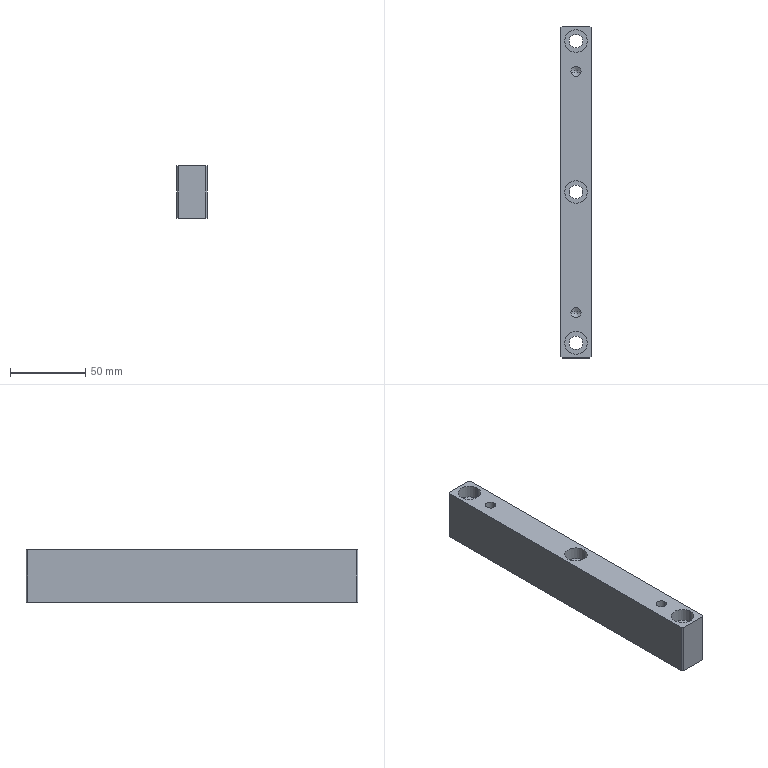Part | SolidWorks | features HoleWzd 2, Chamfer 1, Extrusion 1 | 1 solid | 33 faces | box 20 x 220 x 35 mm | volume 142848 mm3 | cylinder 16 | plane 13 | cone 4 | commonest cylinder face diameters 9 x6 15 x6 6.8 x4
STEP:
#1=CARTESIAN_POINT('',(-3.4,80.,-2.25));
#2=VERTEX_POINT('',#1);
#3=CARTESIAN_POINT('',(3.4,80.,-2.25));
#4=VERTEX_POINT('',#3);
#5=CARTESIAN_POINT('',(0.,80.,-2.25));
#6=DIRECTION('',(0.,0.,1.));
#7=DIRECTION('',(1.,0.,0.));
#8=AXIS2_PLACEMENT_3D('',#5,#6,#7);
#9=CIRCLE('',#8,3.4);
#10=EDGE_CURVE('',#2,#4,#9,.T.);
#11=ORIENTED_EDGE('',*,*,#10,.F.);
#12=CARTESIAN_POINT('',(-3.4,80.,17.5));
#13=VERTEX_POINT('',#12);
#14=CARTESIAN_POINT('',(-3.4,80.,17.5));
#15=DIRECTION('',(0.,0.,1.));
#16=VECTOR('',#15,1000.);
#17=LINE('',#14,#16);
#18=EDGE_CURVE('',#2,#13,#17,.T.);
#19=ORIENTED_EDGE('',*,*,#18,.T.);
#20=CARTESIAN_POINT('',(3.4,80.,17.5));
#21=VERTEX_POINT('',#20);
#22=CARTESIAN_POINT('',(0.,80.,17.5));
#23=DIRECTION('',(0.,0.,1.));
#24=DIRECTION('',(1.,0.,0.));
#25=AXIS2_PLACEMENT_3D('',#22,#23,#24);
#26=CIRCLE('',#25,3.4);
#27=EDGE_CURVE('',#13,#21,#26,.T.);
#28=ORIENTED_EDGE('',*,*,#27,.T.);
#29=CARTESIAN_POINT('',(3.4,80.,17.5));
#30=DIRECTION('',(0.,0.,1.));
#31=VECTOR('',#30,1000.);
#32=LINE('',#29,#31);
#33=EDGE_CURVE('',#4,#21,#32,.T.);
#34=ORIENTED_EDGE('',*,*,#33,.F.);
#35=EDGE_LOOP('',(#11,#19,#28,#34));
#36=FACE_OUTER_BOUND('',#35,.T.);
#37=CARTESIAN_POINT('',(0.,80.,17.5));
#38=DIRECTION('',(0.,0.,1.));
#39=DIRECTION('',(1.,0.,0.));
#40=AXIS2_PLACEMENT_3D('',#37,#38,#39);
#41=CYLINDRICAL_SURFACE('',#40,3.4);
#42=ADVANCED_FACE('',(#36),#41,.F.);
#43=CARTESIAN_POINT('',(0.,80.,-4.293));
#44=VERTEX_POINT('',#43);
#45=CARTESIAN_POINT('',(3.4,80.,-2.25));
#46=DIRECTION('',(0.8572,0.,0.515));
#47=VECTOR('',#46,1000.);
#48=LINE('',#45,#47);
#49=EDGE_CURVE('',#44,#4,#48,.T.);
#50=ORIENTED_EDGE('',*,*,#49,.F.);
#51=CARTESIAN_POINT('',(-3.4,80.,-2.25));
#52=DIRECTION('',(-0.8572,0.,0.515));
#53=VECTOR('',#52,1000.);
#54=LINE('',#51,#53);
#55=EDGE_CURVE('',#44,#2,#54,.T.);
#56=ORIENTED_EDGE('',*,*,#55,.T.);
#57=ORIENTED_EDGE('',*,*,#10,.T.);
#58=EDGE_LOOP('',(#50,#56,#57));
#59=FACE_OUTER_BOUND('',#58,.T.);
#60=CARTESIAN_POINT('',(0.,80.,-2.25));
#61=DIRECTION('',(0.,0.,1.));
#62=DIRECTION('',(1.,0.,0.));
#63=AXIS2_PLACEMENT_3D('',#60,#61,#62);
#64=CONICAL_SURFACE('',#63,3.4,1.03);
#65=ADVANCED_FACE('',(#59),#64,.F.);
#66=CARTESIAN_POINT('',(-3.4,-80.,-2.25));
#67=VERTEX_POINT('',#66);
#68=CARTESIAN_POINT('',(3.4,-80.,-2.25));
#69=VERTEX_POINT('',#68);
#70=CARTESIAN_POINT('',(0.,-80.,-2.25));
#71=DIRECTION('',(0.,0.,1.));
#72=DIRECTION('',(1.,0.,0.));
#73=AXIS2_PLACEMENT_3D('',#70,#71,#72);
#74=CIRCLE('',#73,3.4);
#75=EDGE_CURVE('',#67,#69,#74,.T.);
#76=ORIENTED_EDGE('',*,*,#75,.F.);
#77=CARTESIAN_POINT('',(-3.4,-80.,17.5));
#78=VERTEX_POINT('',#77);
#79=CARTESIAN_POINT('',(-3.4,-80.,17.5));
#80=DIRECTION('',(0.,0.,1.));
#81=VECTOR('',#80,1000.);
#82=LINE('',#79,#81);
#83=EDGE_CURVE('',#67,#78,#82,.T.);
#84=ORIENTED_EDGE('',*,*,#83,.T.);
#85=CARTESIAN_POINT('',(3.4,-80.,17.5));
#86=VERTEX_POINT('',#85);
#87=CARTESIAN_POINT('',(0.,-80.,17.5));
#88=DIRECTION('',(0.,0.,1.));
#89=DIRECTION('',(1.,0.,0.));
#90=AXIS2_PLACEMENT_3D('',#87,#88,#89);
#91=CIRCLE('',#90,3.4);
#92=EDGE_CURVE('',#78,#86,#91,.T.);
#93=ORIENTED_EDGE('',*,*,#92,.T.);
#94=CARTESIAN_POINT('',(3.4,-80.,17.5));
#95=DIRECTION('',(0.,0.,1.));
#96=VECTOR('',#95,1000.);
#97=LINE('',#94,#96);
#98=EDGE_CURVE('',#69,#86,#97,.T.);
#99=ORIENTED_EDGE('',*,*,#98,.F.);
#100=EDGE_LOOP('',(#76,#84,#93,#99));
#101=FACE_OUTER_BOUND('',#100,.T.);
#102=CARTESIAN_POINT('',(0.,-80.,17.5));
#103=DIRECTION('',(0.,0.,1.));
#104=DIRECTION('',(1.,0.,0.));
#105=AXIS2_PLACEMENT_3D('',#102,#103,#104);
#106=CYLINDRICAL_SURFACE('',#105,3.4);
#107=ADVANCED_FACE('',(#101),#106,.F.);
#108=CARTESIAN_POINT('',(0.,-80.,-4.293));
#109=VERTEX_POINT('',#108);
#110=CARTESIAN_POINT('',(3.4,-80.,-2.25));
#111=DIRECTION('',(0.8572,0.,0.515));
#112=VECTOR('',#111,1000.);
#113=LINE('',#110,#112);
#114=EDGE_CURVE('',#109,#69,#113,.T.);
#115=ORIENTED_EDGE('',*,*,#114,.F.);
#116=CARTESIAN_POINT('',(-3.4,-80.,-2.25));
#117=DIRECTION('',(-0.8572,0.,0.515));
#118=VECTOR('',#117,1000.);
#119=LINE('',#116,#118);
#120=EDGE_CURVE('',#109,#67,#119,.T.);
#121=ORIENTED_EDGE('',*,*,#120,.T.);
#122=ORIENTED_EDGE('',*,*,#75,.T.);
#123=EDGE_LOOP('',(#115,#121,#122));
#124=FACE_OUTER_BOUND('',#123,.T.);
#125=CARTESIAN_POINT('',(0.,-80.,-2.25));
#126=DIRECTION('',(0.,0.,1.));
#127=DIRECTION('',(1.,0.,0.));
#128=AXIS2_PLACEMENT_3D('',#125,#126,#127);
#129=CONICAL_SURFACE('',#128,3.4,1.03);
#130=ADVANCED_FACE('',(#124),#129,.F.);
#131=CARTESIAN_POINT('',(-7.5,100.,8.9));
#132=VERTEX_POINT('',#131);
#133=CARTESIAN_POINT('',(7.5,100.,8.9));
#134=VERTEX_POINT('',#133);
#135=CARTESIAN_POINT('',(0.,100.,8.9));
#136=DIRECTION('',(0.,0.,1.));
#137=DIRECTION('',(1.,0.,0.));
#138=AXIS2_PLACEMENT_3D('',#135,#136,#137);
#139=CIRCLE('',#138,7.5);
#140=EDGE_CURVE('',#132,#134,#139,.T.);
#141=ORIENTED_EDGE('',*,*,#140,.F.);
#142=CARTESIAN_POINT('',(-7.5,100.,17.5));
#143=VERTEX_POINT('',#142);
#144=CARTESIAN_POINT('',(-7.5,100.,17.5));
#145=DIRECTION('',(0.,0.,1.));
#146=VECTOR('',#145,1000.);
#147=LINE('',#144,#146);
#148=EDGE_CURVE('',#132,#143,#147,.T.);
#149=ORIENTED_EDGE('',*,*,#148,.T.);
#150=CARTESIAN_POINT('',(7.5,100.,17.5));
#151=VERTEX_POINT('',#150);
#152=CARTESIAN_POINT('',(0.,100.,17.5));
#153=DIRECTION('',(0.,0.,1.));
#154=DIRECTION('',(1.,0.,0.));
#155=AXIS2_PLACEMENT_3D('',#152,#153,#154);
#156=CIRCLE('',#155,7.5);
#157=EDGE_CURVE('',#143,#151,#156,.T.);
#158=ORIENTED_EDGE('',*,*,#157,.T.);
#159=CARTESIAN_POINT('',(7.5,100.,17.5));
#160=DIRECTION('',(0.,0.,1.));
#161=VECTOR('',#160,1000.);
#162=LINE('',#159,#161);
#163=EDGE_CURVE('',#134,#151,#162,.T.);
#164=ORIENTED_EDGE('',*,*,#163,.F.);
#165=EDGE_LOOP('',(#141,#149,#158,#164));
#166=FACE_OUTER_BOUND('',#165,.T.);
#167=CARTESIAN_POINT('',(0.,100.,17.5));
#168=DIRECTION('',(0.,0.,1.));
#169=DIRECTION('',(1.,0.,0.));
#170=AXIS2_PLACEMENT_3D('',#167,#168,#169);
#171=CYLINDRICAL_SURFACE('',#170,7.5);
#172=ADVANCED_FACE('',(#166),#171,.F.);
#173=CARTESIAN_POINT('',(-4.5,100.,-17.5));
#174=VERTEX_POINT('',#173);
#175=CARTESIAN_POINT('',(4.5,100.,-17.5));
#176=VERTEX_POINT('',#175);
#177=CARTESIAN_POINT('',(0.,100.,-17.5));
#178=DIRECTION('',(0.,0.,1.));
#179=DIRECTION('',(1.,0.,0.));
#180=AXIS2_PLACEMENT_3D('',#177,#178,#179);
#181=CIRCLE('',#180,4.5);
#182=EDGE_CURVE('',#174,#176,#181,.T.);
#183=ORIENTED_EDGE('',*,*,#182,.F.);
#184=CARTESIAN_POINT('',(-4.5,100.,8.9));
#185=VERTEX_POINT('',#184);
#186=CARTESIAN_POINT('',(-4.5,100.,17.5));
#187=DIRECTION('',(0.,0.,1.));
#188=VECTOR('',#187,1000.);
#189=LINE('',#186,#188);
#190=EDGE_CURVE('',#174,#185,#189,.T.);
#191=ORIENTED_EDGE('',*,*,#190,.T.);
#192=CARTESIAN_POINT('',(4.5,100.,8.9));
#193=VERTEX_POINT('',#192);
#194=CARTESIAN_POINT('',(0.,100.,8.9));
#195=DIRECTION('',(0.,0.,1.));
#196=DIRECTION('',(1.,0.,0.));
#197=AXIS2_PLACEMENT_3D('',#194,#195,#196);
#198=CIRCLE('',#197,4.5);
#199=EDGE_CURVE('',#185,#193,#198,.T.);
#200=ORIENTED_EDGE('',*,*,#199,.T.);
#201=CARTESIAN_POINT('',(4.5,100.,17.5));
#202=DIRECTION('',(0.,0.,1.));
#203=VECTOR('',#202,1000.);
#204=LINE('',#201,#203);
#205=EDGE_CURVE('',#176,#193,#204,.T.);
#206=ORIENTED_EDGE('',*,*,#205,.F.);
#207=EDGE_LOOP('',(#183,#191,#200,#206));
#208=FACE_OUTER_BOUND('',#207,.T.);
#209=CARTESIAN_POINT('',(0.,100.,17.5));
#210=DIRECTION('',(0.,0.,1.));
#211=DIRECTION('',(1.,0.,0.));
#212=AXIS2_PLACEMENT_3D('',#209,#210,#211);
#213=CYLINDRICAL_SURFACE('',#212,4.5);
#214=ADVANCED_FACE('',(#208),#213,.F.);
#215=CARTESIAN_POINT('',(-7.5,0.,8.9));
#216=VERTEX_POINT('',#215);
#217=CARTESIAN_POINT('',(7.5,0.,8.9));
#218=VERTEX_POINT('',#217);
#219=CARTESIAN_POINT('',(0.,0.,8.9));
#220=DIRECTION('',(0.,0.,1.));
#221=DIRECTION('',(1.,0.,0.));
#222=AXIS2_PLACEMENT_3D('',#219,#220,#221);
#223=CIRCLE('',#222,7.5);
#224=EDGE_CURVE('',#216,#218,#223,.T.);
#225=ORIENTED_EDGE('',*,*,#224,.F.);
#226=CARTESIAN_POINT('',(-7.5,0.,17.5));
#227=VERTEX_POINT('',#226);
#228=CARTESIAN_POINT('',(-7.5,0.,17.5));
#229=DIRECTION('',(0.,0.,1.));
#230=VECTOR('',#229,1000.);
#231=LINE('',#228,#230);
#232=EDGE_CURVE('',#216,#227,#231,.T.);
#233=ORIENTED_EDGE('',*,*,#232,.T.);
#234=CARTESIAN_POINT('',(7.5,0.,17.5));
#235=VERTEX_POINT('',#234);
#236=CARTESIAN_POINT('',(0.,0.,17.5));
#237=DIRECTION('',(0.,0.,1.));
#238=DIRECTION('',(1.,0.,0.));
#239=AXIS2_PLACEMENT_3D('',#236,#237,#238);
#240=CIRCLE('',#239,7.5);
#241=EDGE_CURVE('',#227,#235,#240,.T.);
#242=ORIENTED_EDGE('',*,*,#241,.T.);
#243=CARTESIAN_POINT('',(7.5,0.,17.5));
#244=DIRECTION('',(0.,0.,1.));
#245=VECTOR('',#244,1000.);
#246=LINE('',#243,#245);
#247=EDGE_CURVE('',#218,#235,#246,.T.);
#248=ORIENTED_EDGE('',*,*,#247,.F.);
#249=EDGE_LOOP('',(#225,#233,#242,#248));
#250=FACE_OUTER_BOUND('',#249,.T.);
#251=CARTESIAN_POINT('',(0.,0.,17.5));
#252=DIRECTION('',(0.,0.,1.));
#253=DIRECTION('',(1.,0.,0.));
#254=AXIS2_PLACEMENT_3D('',#251,#252,#253);
#255=CYLINDRICAL_SURFACE('',#254,7.5);
#256=ADVANCED_FACE('',(#250),#255,.F.);
#257=CARTESIAN_POINT('',(-4.5,0.,-17.5));
#258=VERTEX_POINT('',#257);
#259=CARTESIAN_POINT('',(4.5,0.,-17.5));
#260=VERTEX_POINT('',#259);
#261=CARTESIAN_POINT('',(0.,0.,-17.5));
#262=DIRECTION('',(0.,0.,1.));
#263=DIRECTION('',(1.,0.,0.));
#264=AXIS2_PLACEMENT_3D('',#261,#262,#263);
#265=CIRCLE('',#264,4.5);
#266=EDGE_CURVE('',#258,#260,#265,.T.);
#267=ORIENTED_EDGE('',*,*,#266,.F.);
#268=CARTESIAN_POINT('',(-4.5,0.,8.9));
#269=VERTEX_POINT('',#268);
#270=CARTESIAN_POINT('',(-4.5,0.,17.5));
#271=DIRECTION('',(0.,0.,1.));
#272=VECTOR('',#271,1000.);
#273=LINE('',#270,#272);
#274=EDGE_CURVE('',#258,#269,#273,.T.);
#275=ORIENTED_EDGE('',*,*,#274,.T.);
#276=CARTESIAN_POINT('',(4.5,0.,8.9));
#277=VERTEX_POINT('',#276);
#278=CARTESIAN_POINT('',(0.,0.,8.9));
#279=DIRECTION('',(0.,0.,1.));
#280=DIRECTION('',(1.,0.,0.));
#281=AXIS2_PLACEMENT_3D('',#278,#279,#280);
#282=CIRCLE('',#281,4.5);
#283=EDGE_CURVE('',#269,#277,#282,.T.);
#284=ORIENTED_EDGE('',*,*,#283,.T.);
#285=CARTESIAN_POINT('',(4.5,0.,17.5));
#286=DIRECTION('',(0.,0.,1.));
#287=VECTOR('',#286,1000.);
#288=LINE('',#285,#287);
#289=EDGE_CURVE('',#260,#277,#288,.T.);
#290=ORIENTED_EDGE('',*,*,#289,.F.);
#291=EDGE_LOOP('',(#267,#275,#284,#290));
#292=FACE_OUTER_BOUND('',#291,.T.);
#293=CARTESIAN_POINT('',(0.,0.,17.5));
#294=DIRECTION('',(0.,0.,1.));
#295=DIRECTION('',(1.,0.,0.));
#296=AXIS2_PLACEMENT_3D('',#293,#294,#295);
#297=CYLINDRICAL_SURFACE('',#296,4.5);
#298=ADVANCED_FACE('',(#292),#297,.F.);
#299=CARTESIAN_POINT('',(-7.5,-100.,8.9));
#300=VERTEX_POINT('',#299);
#301=CARTESIAN_POINT('',(7.5,-100.,8.9));
#302=VERTEX_POINT('',#301);
#303=CARTESIAN_POINT('',(0.,-100.,8.9));
#304=DIRECTION('',(0.,0.,1.));
#305=DIRECTION('',(1.,0.,0.));
#306=AXIS2_PLACEMENT_3D('',#303,#304,#305);
#307=CIRCLE('',#306,7.5);
#308=EDGE_CURVE('',#300,#302,#307,.T.);
#309=ORIENTED_EDGE('',*,*,#308,.F.);
#310=CARTESIAN_POINT('',(-7.5,-100.,17.5));
#311=VERTEX_POINT('',#310);
#312=CARTESIAN_POINT('',(-7.5,-100.,17.5));
#313=DIRECTION('',(0.,0.,1.));
#314=VECTOR('',#313,1000.);
#315=LINE('',#312,#314);
#316=EDGE_CURVE('',#300,#311,#315,.T.);
#317=ORIENTED_EDGE('',*,*,#316,.T.);
#318=CARTESIAN_POINT('',(7.5,-100.,17.5));
#319=VERTEX_POINT('',#318);
#320=CARTESIAN_POINT('',(0.,-100.,17.5));
#321=DIRECTION('',(0.,0.,1.));
#322=DIRECTION('',(1.,0.,0.));
#323=AXIS2_PLACEMENT_3D('',#320,#321,#322);
#324=CIRCLE('',#323,7.5);
#325=EDGE_CURVE('',#311,#319,#324,.T.);
#326=ORIENTED_EDGE('',*,*,#325,.T.);
#327=CARTESIAN_POINT('',(7.5,-100.,17.5));
#328=DIRECTION('',(0.,0.,1.));
#329=VECTOR('',#328,1000.);
#330=LINE('',#327,#329);
#331=EDGE_CURVE('',#302,#319,#330,.T.);
#332=ORIENTED_EDGE('',*,*,#331,.F.);
#333=EDGE_LOOP('',(#309,#317,#326,#332));
#334=FACE_OUTER_BOUND('',#333,.T.);
#335=CARTESIAN_POINT('',(0.,-100.,17.5));
#336=DIRECTION('',(0.,0.,1.));
#337=DIRECTION('',(1.,0.,0.));
#338=AXIS2_PLACEMENT_3D('',#335,#336,#337);
#339=CYLINDRICAL_SURFACE('',#338,7.5);
#340=ADVANCED_FACE('',(#334),#339,.F.);
#341=CARTESIAN_POINT('',(-4.5,-100.,-17.5));
#342=VERTEX_POINT('',#341);
#343=CARTESIAN_POINT('',(4.5,-100.,-17.5));
#344=VERTEX_POINT('',#343);
#345=CARTESIAN_POINT('',(0.,-100.,-17.5));
#346=DIRECTION('',(0.,0.,1.));
#347=DIRECTION('',(1.,0.,0.));
#348=AXIS2_PLACEMENT_3D('',#345,#346,#347);
#349=CIRCLE('',#348,4.5);
#350=EDGE_CURVE('',#342,#344,#349,.T.);
#351=ORIENTED_EDGE('',*,*,#350,.F.);
#352=CARTESIAN_POINT('',(-4.5,-100.,8.9));
#353=VERTEX_POINT('',#352);
#354=CARTESIAN_POINT('',(-4.5,-100.,17.5));
#355=DIRECTION('',(0.,0.,1.));
#356=VECTOR('',#355,1000.);
#357=LINE('',#354,#356);
#358=EDGE_CURVE('',#342,#353,#357,.T.);
#359=ORIENTED_EDGE('',*,*,#358,.T.);
#360=CARTESIAN_POINT('',(4.5,-100.,8.9));
#361=VERTEX_POINT('',#360);
#362=CARTESIAN_POINT('',(0.,-100.,8.9));
#363=DIRECTION('',(0.,0.,1.));
#364=DIRECTION('',(1.,0.,0.));
#365=AXIS2_PLACEMENT_3D('',#362,#363,#364);
#366=CIRCLE('',#365,4.5);
#367=EDGE_CURVE('',#353,#361,#366,.T.);
#368=ORIENTED_EDGE('',*,*,#367,.T.);
#369=CARTESIAN_POINT('',(4.5,-100.,17.5));
#370=DIRECTION('',(0.,0.,1.));
#371=VECTOR('',#370,1000.);
#372=LINE('',#369,#371);
#373=EDGE_CURVE('',#344,#361,#372,.T.);
#374=ORIENTED_EDGE('',*,*,#373,.F.);
#375=EDGE_LOOP('',(#351,#359,#368,#374));
#376=FACE_OUTER_BOUND('',#375,.T.);
#377=CARTESIAN_POINT('',(0.,-100.,17.5));
#378=DIRECTION('',(0.,0.,1.));
#379=DIRECTION('',(1.,0.,0.));
#380=AXIS2_PLACEMENT_3D('',#377,#378,#379);
#381=CYLINDRICAL_SURFACE('',#380,4.5);
#382=ADVANCED_FACE('',(#376),#381,.F.);
#383=CARTESIAN_POINT('',(10.,-109.,17.5));
#384=VERTEX_POINT('',#383);
#385=CARTESIAN_POINT('',(10.,109.,17.5));
#386=VERTEX_POINT('',#385);
#387=CARTESIAN_POINT('',(10.,-110.,17.5));
#388=DIRECTION('',(0.,1.,0.));
#389=VECTOR('',#388,1000.);
#390=LINE('',#387,#389);
#391=EDGE_CURVE('',#384,#386,#390,.T.);
#392=ORIENTED_EDGE('',*,*,#391,.F.);
#393=CARTESIAN_POINT('',(10.,-109.,-17.5));
#394=VERTEX_POINT('',#393);
#395=CARTESIAN_POINT('',(10.,-109.,17.5));
#396=DIRECTION('',(0.,0.,-1.));
#397=VECTOR('',#396,1000.);
#398=LINE('',#395,#397);
#399=EDGE_CURVE('',#384,#394,#398,.T.);
#400=ORIENTED_EDGE('',*,*,#399,.T.);
#401=CARTESIAN_POINT('',(10.,109.,-17.5));
#402=VERTEX_POINT('',#401);
#403=CARTESIAN_POINT('',(10.,-110.,-17.5));
#404=DIRECTION('',(0.,1.,0.));
#405=VECTOR('',#404,1000.);
#406=LINE('',#403,#405);
#407=EDGE_CURVE('',#394,#402,#406,.T.);
#408=ORIENTED_EDGE('',*,*,#407,.T.);
#409=CARTESIAN_POINT('',(10.,109.,17.5));
#410=DIRECTION('',(0.,0.,1.));
#411=VECTOR('',#410,1000.);
#412=LINE('',#409,#411);
#413=EDGE_CURVE('',#402,#386,#412,.T.);
#414=ORIENTED_EDGE('',*,*,#413,.T.);
#415=EDGE_LOOP('',(#392,#400,#408,#414));
#416=FACE_OUTER_BOUND('',#415,.T.);
#417=CARTESIAN_POINT('',(10.,-110.,17.5));
#418=DIRECTION('',(-1.,0.,0.));
#419=DIRECTION('',(0.,0.,1.));
#420=AXIS2_PLACEMENT_3D('',#417,#418,#419);
#421=PLANE('',#420);
#422=ADVANCED_FACE('',(#416),#421,.F.);
#423=CARTESIAN_POINT('',(9.,110.,17.5));
#424=VERTEX_POINT('',#423);
#425=CARTESIAN_POINT('',(-9.,110.,17.5));
#426=VERTEX_POINT('',#425);
#427=CARTESIAN_POINT('',(-10.,110.,17.5));
#428=DIRECTION('',(-1.,0.,0.));
#429=VECTOR('',#428,1000.);
#430=LINE('',#427,#429);
#431=EDGE_CURVE('',#424,#426,#430,.T.);
#432=ORIENTED_EDGE('',*,*,#431,.F.);
#433=CARTESIAN_POINT('',(9.,110.,-17.5));
#434=VERTEX_POINT('',#433);
#435=CARTESIAN_POINT('',(9.,110.,17.5));
#436=DIRECTION('',(0.,0.,-1.));
#437=VECTOR('',#436,1000.);
#438=LINE('',#435,#437);
#439=EDGE_CURVE('',#424,#434,#438,.T.);
#440=ORIENTED_EDGE('',*,*,#439,.T.);
#441=CARTESIAN_POINT('',(-9.,110.,-17.5));
#442=VERTEX_POINT('',#441);
#443=CARTESIAN_POINT('',(-10.,110.,-17.5));
#444=DIRECTION('',(-1.,0.,0.));
#445=VECTOR('',#444,1000.);
#446=LINE('',#443,#445);
#447=EDGE_CURVE('',#434,#442,#446,.T.);
#448=ORIENTED_EDGE('',*,*,#447,.T.);
#449=CARTESIAN_POINT('',(-9.,110.,17.5));
#450=DIRECTION('',(0.,0.,1.));
#451=VECTOR('',#450,1000.);
#452=LINE('',#449,#451);
#453=EDGE_CURVE('',#442,#426,#452,.T.);
#454=ORIENTED_EDGE('',*,*,#453,.T.);
#455=EDGE_LOOP('',(#432,#440,#448,#454));
#456=FACE_OUTER_BOUND('',#455,.T.);
#457=CARTESIAN_POINT('',(-10.,110.,17.5));
#458=DIRECTION('',(0.,-1.,0.));
#459=DIRECTION('',(0.,0.,-1.));
#460=AXIS2_PLACEMENT_3D('',#457,#458,#459);
#461=PLANE('',#460);
#462=ADVANCED_FACE('',(#456),#461,.F.);
#463=CARTESIAN_POINT('',(-10.,109.,-17.5));
#464=VERTEX_POINT('',#463);
#465=CARTESIAN_POINT('',(-10.,-109.,-17.5));
#466=VERTEX_POINT('',#465);
#467=CARTESIAN_POINT('',(-10.,-110.,-17.5));
#468=DIRECTION('',(0.,-1.,0.));
#469=VECTOR('',#468,1000.);
#470=LINE('',#467,#469);
#471=EDGE_CURVE('',#464,#466,#470,.T.);
#472=ORIENTED_EDGE('',*,*,#471,.T.);
#473=CARTESIAN_POINT('',(-10.,-109.,17.5));
#474=VERTEX_POINT('',#473);
#475=CARTESIAN_POINT('',(-10.,-109.,17.5));
#476=DIRECTION('',(0.,0.,1.));
#477=VECTOR('',#476,1000.);
#478=LINE('',#475,#477);
#479=EDGE_CURVE('',#466,#474,#478,.T.);
#480=ORIENTED_EDGE('',*,*,#479,.T.);
#481=CARTESIAN_POINT('',(-10.,109.,17.5));
#482=VERTEX_POINT('',#481);
#483=CARTESIAN_POINT('',(-10.,-110.,17.5));
#484=DIRECTION('',(0.,-1.,0.));
#485=VECTOR('',#484,1000.);
#486=LINE('',#483,#485);
#487=EDGE_CURVE('',#482,#474,#486,.T.);
#488=ORIENTED_EDGE('',*,*,#487,.F.);
#489=CARTESIAN_POINT('',(-10.,109.,17.5));
#490=DIRECTION('',(0.,0.,-1.));
#491=VECTOR('',#490,1000.);
#492=LINE('',#489,#491);
#493=EDGE_CURVE('',#482,#464,#492,.T.);
#494=ORIENTED_EDGE('',*,*,#493,.T.);
#495=EDGE_LOOP('',(#472,#480,#488,#494));
#496=FACE_OUTER_BOUND('',#495,.T.);
#497=CARTESIAN_POINT('',(-10.,-110.,17.5));
#498=DIRECTION('',(1.,0.,0.));
#499=DIRECTION('',(0.,0.,-1.));
#500=AXIS2_PLACEMENT_3D('',#497,#498,#499);
#501=PLANE('',#500);
#502=ADVANCED_FACE('',(#496),#501,.F.);
#503=CARTESIAN_POINT('',(-9.,-110.,17.5));
#504=VERTEX_POINT('',#503);
#505=CARTESIAN_POINT('',(9.,-110.,17.5));
#506=VERTEX_POINT('',#505);
#507=CARTESIAN_POINT('',(-10.,-110.,17.5));
#508=DIRECTION('',(1.,0.,0.));
#509=VECTOR('',#508,1000.);
#510=LINE('',#507,#509);
#511=EDGE_CURVE('',#504,#506,#510,.T.);
#512=ORIENTED_EDGE('',*,*,#511,.F.);
#513=CARTESIAN_POINT('',(-9.,-110.,-17.5));
#514=VERTEX_POINT('',#513);
#515=CARTESIAN_POINT('',(-9.,-110.,17.5));
#516=DIRECTION('',(0.,0.,-1.));
#517=VECTOR('',#516,1000.);
#518=LINE('',#515,#517);
#519=EDGE_CURVE('',#504,#514,#518,.T.);
#520=ORIENTED_EDGE('',*,*,#519,.T.);
#521=CARTESIAN_POINT('',(9.,-110.,-17.5));
#522=VERTEX_POINT('',#521);
#523=CARTESIAN_POINT('',(-10.,-110.,-17.5));
#524=DIRECTION('',(1.,0.,0.));
#525=VECTOR('',#524,1000.);
#526=LINE('',#523,#525);
#527=EDGE_CURVE('',#514,#522,#526,.T.);
#528=ORIENTED_EDGE('',*,*,#527,.T.);
#529=CARTESIAN_POINT('',(9.,-110.,17.5));
#530=DIRECTION('',(0.,0.,1.));
#531=VECTOR('',#530,1000.);
#532=LINE('',#529,#531);
#533=EDGE_CURVE('',#522,#506,#532,.T.);
#534=ORIENTED_EDGE('',*,*,#533,.T.);
#535=EDGE_LOOP('',(#512,#520,#528,#534));
#536=FACE_OUTER_BOUND('',#535,.T.);
#537=CARTESIAN_POINT('',(-10.,-110.,17.5));
#538=DIRECTION('',(0.,1.,0.));
#539=DIRECTION('',(0.,0.,1.));
#540=AXIS2_PLACEMENT_3D('',#537,#538,#539);
#541=PLANE('',#540);
#542=ADVANCED_FACE('',(#536),#541,.F.);
#543=CARTESIAN_POINT('',(0.,80.,17.5));
#544=DIRECTION('',(0.,0.,1.));
#545=DIRECTION('',(1.,0.,0.));
#546=AXIS2_PLACEMENT_3D('',#543,#544,#545);
#547=CIRCLE('',#546,3.4);
#548=EDGE_CURVE('',#21,#13,#547,.T.);
#549=ORIENTED_EDGE('',*,*,#548,.F.);
#550=ORIENTED_EDGE('',*,*,#27,.F.);
#551=EDGE_LOOP('',(#549,#550));
#552=FACE_BOUND('',#551,.T.);
#553=CARTESIAN_POINT('',(0.,-80.,17.5));
#554=DIRECTION('',(0.,0.,1.));
#555=DIRECTION('',(1.,0.,0.));
#556=AXIS2_PLACEMENT_3D('',#553,#554,#555);
#557=CIRCLE('',#556,3.4);
#558=EDGE_CURVE('',#86,#78,#557,.T.);
#559=ORIENTED_EDGE('',*,*,#558,.F.);
#560=ORIENTED_EDGE('',*,*,#92,.F.);
#561=EDGE_LOOP('',(#559,#560));
#562=FACE_BOUND('',#561,.T.);
#563=CARTESIAN_POINT('',(0.,100.,17.5));
#564=DIRECTION('',(0.,0.,1.));
#565=DIRECTION('',(1.,0.,0.));
#566=AXIS2_PLACEMENT_3D('',#563,#564,#565);
#567=CIRCLE('',#566,7.5);
#568=EDGE_CURVE('',#151,#143,#567,.T.);
#569=ORIENTED_EDGE('',*,*,#568,.F.);
#570=ORIENTED_EDGE('',*,*,#157,.F.);
#571=EDGE_LOOP('',(#569,#570));
#572=FACE_BOUND('',#571,.T.);
#573=CARTESIAN_POINT('',(0.,0.,17.5));
#574=DIRECTION('',(0.,0.,1.));
#575=DIRECTION('',(1.,0.,0.));
#576=AXIS2_PLACEMENT_3D('',#573,#574,#575);
#577=CIRCLE('',#576,7.5);
#578=EDGE_CURVE('',#235,#227,#577,.T.);
#579=ORIENTED_EDGE('',*,*,#578,.F.);
#580=ORIENTED_EDGE('',*,*,#241,.F.);
#581=EDGE_LOOP('',(#579,#580));
#582=FACE_BOUND('',#581,.T.);
#583=CARTESIAN_POINT('',(0.,-100.,17.5));
#584=DIRECTION('',(0.,0.,1.));
#585=DIRECTION('',(1.,0.,0.));
#586=AXIS2_PLACEMENT_3D('',#583,#584,#585);
#587=CIRCLE('',#586,7.5);
#588=EDGE_CURVE('',#319,#311,#587,.T.);
#589=ORIENTED_EDGE('',*,*,#588,.F.);
#590=ORIENTED_EDGE('',*,*,#325,.F.);
#591=EDGE_LOOP('',(#589,#590));
#592=FACE_BOUND('',#591,.T.);
#593=ORIENTED_EDGE('',*,*,#487,.T.);
#594=CARTESIAN_POINT('',(-9.,-110.,17.5));
#595=DIRECTION('',(0.7071,-0.7071,0.));
#596=VECTOR('',#595,1000.);
#597=LINE('',#594,#596);
#598=EDGE_CURVE('',#474,#504,#597,.T.);
#599=ORIENTED_EDGE('',*,*,#598,.T.);
#600=ORIENTED_EDGE('',*,*,#511,.T.);
#601=CARTESIAN_POINT('',(10.,-109.,17.5));
#602=DIRECTION('',(0.7071,0.7071,0.));
#603=VECTOR('',#602,1000.);
#604=LINE('',#601,#603);
#605=EDGE_CURVE('',#506,#384,#604,.T.);
#606=ORIENTED_EDGE('',*,*,#605,.T.);
#607=ORIENTED_EDGE('',*,*,#391,.T.);
#608=CARTESIAN_POINT('',(9.,110.,17.5));
#609=DIRECTION('',(-0.7071,0.7071,0.));
#610=VECTOR('',#609,1000.);
#611=LINE('',#608,#610);
#612=EDGE_CURVE('',#386,#424,#611,.T.);
#613=ORIENTED_EDGE('',*,*,#612,.T.);
#614=ORIENTED_EDGE('',*,*,#431,.T.);
#615=CARTESIAN_POINT('',(-10.,109.,17.5));
#616=DIRECTION('',(-0.7071,-0.7071,0.));
#617=VECTOR('',#616,1000.);
#618=LINE('',#615,#617);
#619=EDGE_CURVE('',#426,#482,#618,.T.);
#620=ORIENTED_EDGE('',*,*,#619,.T.);
#621=EDGE_LOOP('',(#593,#599,#600,#606,#607,#613,#614,#620));
#622=FACE_OUTER_BOUND('',#621,.T.);
#623=CARTESIAN_POINT('',(0.,0.,17.5));
#624=DIRECTION('',(0.,0.,-1.));
#625=DIRECTION('',(-1.,0.,0.));
#626=AXIS2_PLACEMENT_3D('',#623,#624,#625);
#627=PLANE('',#626);
#628=ADVANCED_FACE('',(#552,#562,#572,#582,#592,#622),#627,.F.);
#629=CARTESIAN_POINT('',(0.,100.,-17.5));
#630=DIRECTION('',(0.,0.,1.));
#631=DIRECTION('',(1.,0.,0.));
#632=AXIS2_PLACEMENT_3D('',#629,#630,#631);
#633=CIRCLE('',#632,4.5);
#634=EDGE_CURVE('',#176,#174,#633,.T.);
#635=ORIENTED_EDGE('',*,*,#634,.T.);
#636=ORIENTED_EDGE('',*,*,#182,.T.);
#637=EDGE_LOOP('',(#635,#636));
#638=FACE_BOUND('',#637,.T.);
#639=CARTESIAN_POINT('',(0.,0.,-17.5));
#640=DIRECTION('',(0.,0.,1.));
#641=DIRECTION('',(1.,0.,0.));
#642=AXIS2_PLACEMENT_3D('',#639,#640,#641);
#643=CIRCLE('',#642,4.5);
#644=EDGE_CURVE('',#260,#258,#643,.T.);
#645=ORIENTED_EDGE('',*,*,#644,.T.);
#646=ORIENTED_EDGE('',*,*,#266,.T.);
#647=EDGE_LOOP('',(#645,#646));
#648=FACE_BOUND('',#647,.T.);
#649=CARTESIAN_POINT('',(0.,-100.,-17.5));
#650=DIRECTION('',(0.,0.,1.));
#651=DIRECTION('',(1.,0.,0.));
#652=AXIS2_PLACEMENT_3D('',#649,#650,#651);
#653=CIRCLE('',#652,4.5);
#654=EDGE_CURVE('',#344,#342,#653,.T.);
#655=ORIENTED_EDGE('',*,*,#654,.T.);
#656=ORIENTED_EDGE('',*,*,#350,.T.);
#657=EDGE_LOOP('',(#655,#656));
#658=FACE_BOUND('',#657,.T.);
#659=ORIENTED_EDGE('',*,*,#527,.F.);
#660=CARTESIAN_POINT('',(-59.5,-59.5,-17.5));
#661=DIRECTION('',(-0.7071,0.7071,0.));
#662=VECTOR('',#661,1000.);
#663=LINE('',#660,#662);
#664=EDGE_CURVE('',#514,#466,#663,.T.);
#665=ORIENTED_EDGE('',*,*,#664,.T.);
#666=ORIENTED_EDGE('',*,*,#471,.F.);
#667=CARTESIAN_POINT('',(-59.5,59.5,-17.5));
#668=DIRECTION('',(0.7071,0.7071,0.));
#669=VECTOR('',#668,1000.);
#670=LINE('',#667,#669);
#671=EDGE_CURVE('',#464,#442,#670,.T.);
#672=ORIENTED_EDGE('',*,*,#671,.T.);
#673=ORIENTED_EDGE('',*,*,#447,.F.);
#674=CARTESIAN_POINT('',(59.5,59.5,-17.5));
#675=DIRECTION('',(0.7071,-0.7071,0.));
#676=VECTOR('',#675,1000.);
#677=LINE('',#674,#676);
#678=EDGE_CURVE('',#434,#402,#677,.T.);
#679=ORIENTED_EDGE('',*,*,#678,.T.);
#680=ORIENTED_EDGE('',*,*,#407,.F.);
#681=CARTESIAN_POINT('',(59.5,-59.5,-17.5));
#682=DIRECTION('',(-0.7071,-0.7071,0.));
#683=VECTOR('',#682,1000.);
#684=LINE('',#681,#683);
#685=EDGE_CURVE('',#394,#522,#684,.T.);
#686=ORIENTED_EDGE('',*,*,#685,.T.);
#687=EDGE_LOOP('',(#659,#665,#666,#672,#673,#679,#680,#686));
#688=FACE_OUTER_BOUND('',#687,.T.);
#689=CARTESIAN_POINT('',(0.,0.,-17.5));
#690=DIRECTION('',(0.,0.,-1.));
#691=DIRECTION('',(-1.,0.,0.));
#692=AXIS2_PLACEMENT_3D('',#689,#690,#691);
#693=PLANE('',#692);
#694=ADVANCED_FACE('',(#638,#648,#658,#688),#693,.T.);
#695=ORIENTED_EDGE('',*,*,#358,.F.);
#696=ORIENTED_EDGE('',*,*,#654,.F.);
#697=ORIENTED_EDGE('',*,*,#373,.T.);
#698=CARTESIAN_POINT('',(0.,-100.,8.9));
#699=DIRECTION('',(0.,0.,1.));
#700=DIRECTION('',(1.,0.,0.));
#701=AXIS2_PLACEMENT_3D('',#698,#699,#700);
#702=CIRCLE('',#701,4.5);
#703=EDGE_CURVE('',#361,#353,#702,.T.);
#704=ORIENTED_EDGE('',*,*,#703,.T.);
#705=EDGE_LOOP('',(#695,#696,#697,#704));
#706=FACE_OUTER_BOUND('',#705,.T.);
#707=CARTESIAN_POINT('',(0.,-100.,17.5));
#708=DIRECTION('',(0.,0.,1.));
#709=DIRECTION('',(1.,0.,0.));
#710=AXIS2_PLACEMENT_3D('',#707,#708,#709);
#711=CYLINDRICAL_SURFACE('',#710,4.5);
#712=ADVANCED_FACE('',(#706),#711,.F.);
#713=ORIENTED_EDGE('',*,*,#703,.F.);
#714=ORIENTED_EDGE('',*,*,#367,.F.);
#715=EDGE_LOOP('',(#713,#714));
#716=FACE_BOUND('',#715,.T.);
#717=CARTESIAN_POINT('',(0.,-100.,8.9));
#718=DIRECTION('',(0.,0.,1.));
#719=DIRECTION('',(1.,0.,0.));
#720=AXIS2_PLACEMENT_3D('',#717,#718,#719);
#721=CIRCLE('',#720,7.5);
#722=EDGE_CURVE('',#302,#300,#721,.T.);
#723=ORIENTED_EDGE('',*,*,#722,.T.);
#724=ORIENTED_EDGE('',*,*,#308,.T.);
#725=EDGE_LOOP('',(#723,#724));
#726=FACE_OUTER_BOUND('',#725,.T.);
#727=CARTESIAN_POINT('',(4.5,-100.,8.9));
#728=DIRECTION('',(0.,0.,-1.));
#729=DIRECTION('',(-1.,0.,0.));
#730=AXIS2_PLACEMENT_3D('',#727,#728,#729);
#731=PLANE('',#730);
#732=ADVANCED_FACE('',(#716,#726),#731,.F.);
#733=ORIENTED_EDGE('',*,*,#316,.F.);
#734=ORIENTED_EDGE('',*,*,#722,.F.);
#735=ORIENTED_EDGE('',*,*,#331,.T.);
#736=ORIENTED_EDGE('',*,*,#588,.T.);
#737=EDGE_LOOP('',(#733,#734,#735,#736));
#738=FACE_OUTER_BOUND('',#737,.T.);
#739=CARTESIAN_POINT('',(0.,-100.,17.5));
#740=DIRECTION('',(0.,0.,1.));
#741=DIRECTION('',(1.,0.,0.));
#742=AXIS2_PLACEMENT_3D('',#739,#740,#741);
#743=CYLINDRICAL_SURFACE('',#742,7.5);
#744=ADVANCED_FACE('',(#738),#743,.F.);
#745=ORIENTED_EDGE('',*,*,#274,.F.);
#746=ORIENTED_EDGE('',*,*,#644,.F.);
#747=ORIENTED_EDGE('',*,*,#289,.T.);
#748=CARTESIAN_POINT('',(0.,0.,8.9));
#749=DIRECTION('',(0.,0.,1.));
#750=DIRECTION('',(1.,0.,0.));
#751=AXIS2_PLACEMENT_3D('',#748,#749,#750);
#752=CIRCLE('',#751,4.5);
#753=EDGE_CURVE('',#277,#269,#752,.T.);
#754=ORIENTED_EDGE('',*,*,#753,.T.);
#755=EDGE_LOOP('',(#745,#746,#747,#754));
#756=FACE_OUTER_BOUND('',#755,.T.);
#757=CARTESIAN_POINT('',(0.,0.,17.5));
#758=DIRECTION('',(0.,0.,1.));
#759=DIRECTION('',(1.,0.,0.));
#760=AXIS2_PLACEMENT_3D('',#757,#758,#759);
#761=CYLINDRICAL_SURFACE('',#760,4.5);
#762=ADVANCED_FACE('',(#756),#761,.F.);
#763=ORIENTED_EDGE('',*,*,#753,.F.);
#764=ORIENTED_EDGE('',*,*,#283,.F.);
#765=EDGE_LOOP('',(#763,#764));
#766=FACE_BOUND('',#765,.T.);
#767=CARTESIAN_POINT('',(0.,0.,8.9));
#768=DIRECTION('',(0.,0.,1.));
#769=DIRECTION('',(1.,0.,0.));
#770=AXIS2_PLACEMENT_3D('',#767,#768,#769);
#771=CIRCLE('',#770,7.5);
#772=EDGE_CURVE('',#218,#216,#771,.T.);
#773=ORIENTED_EDGE('',*,*,#772,.T.);
#774=ORIENTED_EDGE('',*,*,#224,.T.);
#775=EDGE_LOOP('',(#773,#774));
#776=FACE_OUTER_BOUND('',#775,.T.);
#777=CARTESIAN_POINT('',(4.5,0.,8.9));
#778=DIRECTION('',(0.,0.,-1.));
#779=DIRECTION('',(-1.,0.,0.));
#780=AXIS2_PLACEMENT_3D('',#777,#778,#779);
#781=PLANE('',#780);
#782=ADVANCED_FACE('',(#766,#776),#781,.F.);
#783=ORIENTED_EDGE('',*,*,#232,.F.);
#784=ORIENTED_EDGE('',*,*,#772,.F.);
#785=ORIENTED_EDGE('',*,*,#247,.T.);
#786=ORIENTED_EDGE('',*,*,#578,.T.);
#787=EDGE_LOOP('',(#783,#784,#785,#786));
#788=FACE_OUTER_BOUND('',#787,.T.);
#789=CARTESIAN_POINT('',(0.,0.,17.5));
#790=DIRECTION('',(0.,0.,1.));
#791=DIRECTION('',(1.,0.,0.));
#792=AXIS2_PLACEMENT_3D('',#789,#790,#791);
#793=CYLINDRICAL_SURFACE('',#792,7.5);
#794=ADVANCED_FACE('',(#788),#793,.F.);
#795=ORIENTED_EDGE('',*,*,#190,.F.);
#796=ORIENTED_EDGE('',*,*,#634,.F.);
#797=ORIENTED_EDGE('',*,*,#205,.T.);
#798=CARTESIAN_POINT('',(0.,100.,8.9));
#799=DIRECTION('',(0.,0.,1.));
#800=DIRECTION('',(1.,0.,0.));
#801=AXIS2_PLACEMENT_3D('',#798,#799,#800);
#802=CIRCLE('',#801,4.5);
#803=EDGE_CURVE('',#193,#185,#802,.T.);
#804=ORIENTED_EDGE('',*,*,#803,.T.);
#805=EDGE_LOOP('',(#795,#796,#797,#804));
#806=FACE_OUTER_BOUND('',#805,.T.);
#807=CARTESIAN_POINT('',(0.,100.,17.5));
#808=DIRECTION('',(0.,0.,1.));
#809=DIRECTION('',(1.,0.,0.));
#810=AXIS2_PLACEMENT_3D('',#807,#808,#809);
#811=CYLINDRICAL_SURFACE('',#810,4.5);
#812=ADVANCED_FACE('',(#806),#811,.F.);
#813=ORIENTED_EDGE('',*,*,#803,.F.);
#814=ORIENTED_EDGE('',*,*,#199,.F.);
#815=EDGE_LOOP('',(#813,#814));
#816=FACE_BOUND('',#815,.T.);
#817=CARTESIAN_POINT('',(0.,100.,8.9));
#818=DIRECTION('',(0.,0.,1.));
#819=DIRECTION('',(1.,0.,0.));
#820=AXIS2_PLACEMENT_3D('',#817,#818,#819);
#821=CIRCLE('',#820,7.5);
#822=EDGE_CURVE('',#134,#132,#821,.T.);
#823=ORIENTED_EDGE('',*,*,#822,.T.);
#824=ORIENTED_EDGE('',*,*,#140,.T.);
#825=EDGE_LOOP('',(#823,#824));
#826=FACE_OUTER_BOUND('',#825,.T.);
#827=CARTESIAN_POINT('',(4.5,100.,8.9));
#828=DIRECTION('',(0.,0.,-1.));
#829=DIRECTION('',(-1.,0.,0.));
#830=AXIS2_PLACEMENT_3D('',#827,#828,#829);
#831=PLANE('',#830);
#832=ADVANCED_FACE('',(#816,#826),#831,.F.);
#833=ORIENTED_EDGE('',*,*,#148,.F.);
#834=ORIENTED_EDGE('',*,*,#822,.F.);
#835=ORIENTED_EDGE('',*,*,#163,.T.);
#836=ORIENTED_EDGE('',*,*,#568,.T.);
#837=EDGE_LOOP('',(#833,#834,#835,#836));
#838=FACE_OUTER_BOUND('',#837,.T.);
#839=CARTESIAN_POINT('',(0.,100.,17.5));
#840=DIRECTION('',(0.,0.,1.));
#841=DIRECTION('',(1.,0.,0.));
#842=AXIS2_PLACEMENT_3D('',#839,#840,#841);
#843=CYLINDRICAL_SURFACE('',#842,7.5);
#844=ADVANCED_FACE('',(#838),#843,.F.);
#845=ORIENTED_EDGE('',*,*,#120,.F.);
#846=ORIENTED_EDGE('',*,*,#114,.T.);
#847=CARTESIAN_POINT('',(0.,-80.,-2.25));
#848=DIRECTION('',(0.,0.,1.));
#849=DIRECTION('',(1.,0.,0.));
#850=AXIS2_PLACEMENT_3D('',#847,#848,#849);
#851=CIRCLE('',#850,3.4);
#852=EDGE_CURVE('',#69,#67,#851,.T.);
#853=ORIENTED_EDGE('',*,*,#852,.T.);
#854=EDGE_LOOP('',(#845,#846,#853));
#855=FACE_OUTER_BOUND('',#854,.T.);
#856=CARTESIAN_POINT('',(0.,-80.,-2.25));
#857=DIRECTION('',(0.,0.,1.));
#858=DIRECTION('',(1.,0.,0.));
#859=AXIS2_PLACEMENT_3D('',#856,#857,#858);
#860=CONICAL_SURFACE('',#859,3.4,1.03);
#861=ADVANCED_FACE('',(#855),#860,.F.);
#862=ORIENTED_EDGE('',*,*,#83,.F.);
#863=ORIENTED_EDGE('',*,*,#852,.F.);
#864=ORIENTED_EDGE('',*,*,#98,.T.);
#865=ORIENTED_EDGE('',*,*,#558,.T.);
#866=EDGE_LOOP('',(#862,#863,#864,#865));
#867=FACE_OUTER_BOUND('',#866,.T.);
#868=CARTESIAN_POINT('',(0.,-80.,17.5));
#869=DIRECTION('',(0.,0.,1.));
#870=DIRECTION('',(1.,0.,0.));
#871=AXIS2_PLACEMENT_3D('',#868,#869,#870);
#872=CYLINDRICAL_SURFACE('',#871,3.4);
#873=ADVANCED_FACE('',(#867),#872,.F.);
#874=ORIENTED_EDGE('',*,*,#55,.F.);
#875=ORIENTED_EDGE('',*,*,#49,.T.);
#876=CARTESIAN_POINT('',(0.,80.,-2.25));
#877=DIRECTION('',(0.,0.,1.));
#878=DIRECTION('',(1.,0.,0.));
#879=AXIS2_PLACEMENT_3D('',#876,#877,#878);
#880=CIRCLE('',#879,3.4);
#881=EDGE_CURVE('',#4,#2,#880,.T.);
#882=ORIENTED_EDGE('',*,*,#881,.T.);
#883=EDGE_LOOP('',(#874,#875,#882));
#884=FACE_OUTER_BOUND('',#883,.T.);
#885=CARTESIAN_POINT('',(0.,80.,-2.25));
#886=DIRECTION('',(0.,0.,1.));
#887=DIRECTION('',(1.,0.,0.));
#888=AXIS2_PLACEMENT_3D('',#885,#886,#887);
#889=CONICAL_SURFACE('',#888,3.4,1.03);
#890=ADVANCED_FACE('',(#884),#889,.F.);
#891=ORIENTED_EDGE('',*,*,#18,.F.);
#892=ORIENTED_EDGE('',*,*,#881,.F.);
#893=ORIENTED_EDGE('',*,*,#33,.T.);
#894=ORIENTED_EDGE('',*,*,#548,.T.);
#895=EDGE_LOOP('',(#891,#892,#893,#894));
#896=FACE_OUTER_BOUND('',#895,.T.);
#897=CARTESIAN_POINT('',(0.,80.,17.5));
#898=DIRECTION('',(0.,0.,1.));
#899=DIRECTION('',(1.,0.,0.));
#900=AXIS2_PLACEMENT_3D('',#897,#898,#899);
#901=CYLINDRICAL_SURFACE('',#900,3.4);
#902=ADVANCED_FACE('',(#896),#901,.F.);
#903=ORIENTED_EDGE('',*,*,#598,.F.);
#904=ORIENTED_EDGE('',*,*,#479,.F.);
#905=ORIENTED_EDGE('',*,*,#664,.F.);
#906=ORIENTED_EDGE('',*,*,#519,.F.);
#907=EDGE_LOOP('',(#903,#904,#905,#906));
#908=FACE_OUTER_BOUND('',#907,.T.);
#909=CARTESIAN_POINT('',(-9.,-110.,17.5));
#910=DIRECTION('',(0.7071,0.7071,0.));
#911=DIRECTION('',(0.,0.,-1.));
#912=AXIS2_PLACEMENT_3D('',#909,#910,#911);
#913=PLANE('',#912);
#914=ADVANCED_FACE('',(#908),#913,.F.);
#915=ORIENTED_EDGE('',*,*,#605,.F.);
#916=ORIENTED_EDGE('',*,*,#533,.F.);
#917=ORIENTED_EDGE('',*,*,#685,.F.);
#918=ORIENTED_EDGE('',*,*,#399,.F.);
#919=EDGE_LOOP('',(#915,#916,#917,#918));
#920=FACE_OUTER_BOUND('',#919,.T.);
#921=CARTESIAN_POINT('',(10.,-109.,17.5));
#922=DIRECTION('',(-0.7071,0.7071,0.));
#923=DIRECTION('',(0.,0.,-1.));
#924=AXIS2_PLACEMENT_3D('',#921,#922,#923);
#925=PLANE('',#924);
#926=ADVANCED_FACE('',(#920),#925,.F.);
#927=ORIENTED_EDGE('',*,*,#612,.F.);
#928=ORIENTED_EDGE('',*,*,#413,.F.);
#929=ORIENTED_EDGE('',*,*,#678,.F.);
#930=ORIENTED_EDGE('',*,*,#439,.F.);
#931=EDGE_LOOP('',(#927,#928,#929,#930));
#932=FACE_OUTER_BOUND('',#931,.T.);
#933=CARTESIAN_POINT('',(9.,110.,17.5));
#934=DIRECTION('',(-0.7071,-0.7071,0.));
#935=DIRECTION('',(0.,0.,-1.));
#936=AXIS2_PLACEMENT_3D('',#933,#934,#935);
#937=PLANE('',#936);
#938=ADVANCED_FACE('',(#932),#937,.F.);
#939=ORIENTED_EDGE('',*,*,#619,.F.);
#940=ORIENTED_EDGE('',*,*,#453,.F.);
#941=ORIENTED_EDGE('',*,*,#671,.F.);
#942=ORIENTED_EDGE('',*,*,#493,.F.);
#943=EDGE_LOOP('',(#939,#940,#941,#942));
#944=FACE_OUTER_BOUND('',#943,.T.);
#945=CARTESIAN_POINT('',(-10.,109.,17.5));
#946=DIRECTION('',(0.7071,-0.7071,0.));
#947=DIRECTION('',(0.,0.,-1.));
#948=AXIS2_PLACEMENT_3D('',#945,#946,#947);
#949=PLANE('',#948);
#950=ADVANCED_FACE('',(#944),#949,.F.);
#951=CLOSED_SHELL('',(#42,#65,#107,#130,#172,#214,#256,#298,#340,#382,#422,#462,#502,#542,#628,#694,#712,#732,#744,#762,#782,#794,#812,#832,#844,#861,#873,#890,#902,#914,#926,#938,#950));
#952=MANIFOLD_SOLID_BREP('',#951);
#953=CARTESIAN_POINT('',(0.,0.,0.));
#954=DIRECTION('',(0.,0.,1.));
#955=DIRECTION('',(1.,0.,0.));
#956=AXIS2_PLACEMENT_3D('',#953,#954,#955);
#957=(LENGTH_UNIT()NAMED_UNIT(*)SI_UNIT(.MILLI.,.METRE.));
#958=UNCERTAINTY_MEASURE_WITH_UNIT(LENGTH_MEASURE(0.00001),#957,'','');
#959=(NAMED_UNIT(*)PLANE_ANGLE_UNIT()SI_UNIT($,.RADIAN.));
#960=(NAMED_UNIT(*)SI_UNIT($,.STERADIAN.)SOLID_ANGLE_UNIT());
#961=(GEOMETRIC_REPRESENTATION_CONTEXT(3)GLOBAL_UNCERTAINTY_ASSIGNED_CONTEXT((#958))GLOBAL_UNIT_ASSIGNED_CONTEXT((#957,#959,#960))REPRESENTATION_CONTEXT('',''));
#962=ADVANCED_BREP_SHAPE_REPRESENTATION('',(#952,#956),#961);